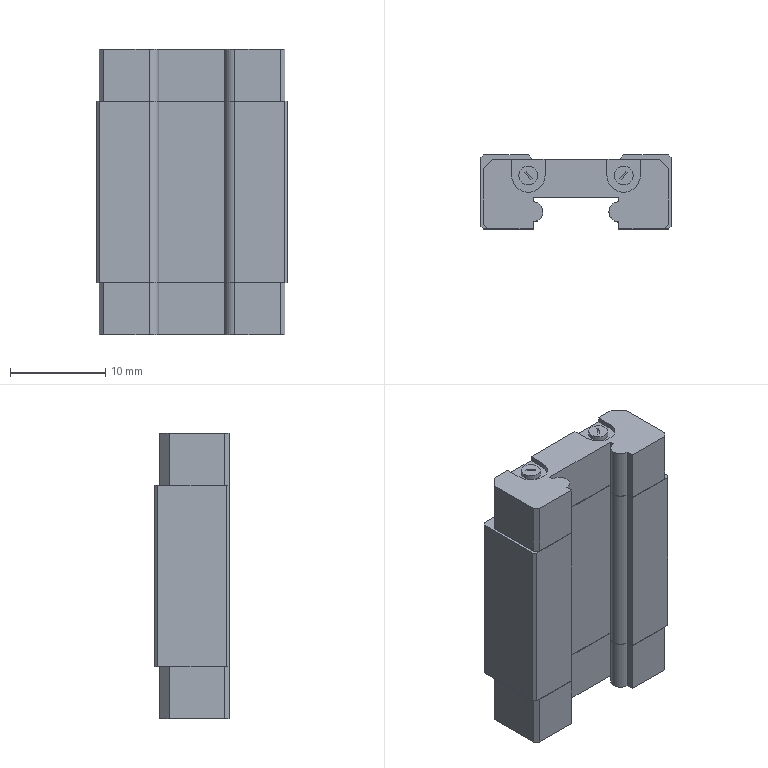Part | STEP file | 11-b_SEB1011 | 1 solid | 167 faces | box 20 x 7.8 x 30 mm | volume 3540 mm3 | plane 116 | cylinder 35 | cone 16 | commonest cylinder face diameters 2.08 x9 2 x8 2.459 x8 2.04 x6 3.5 x4